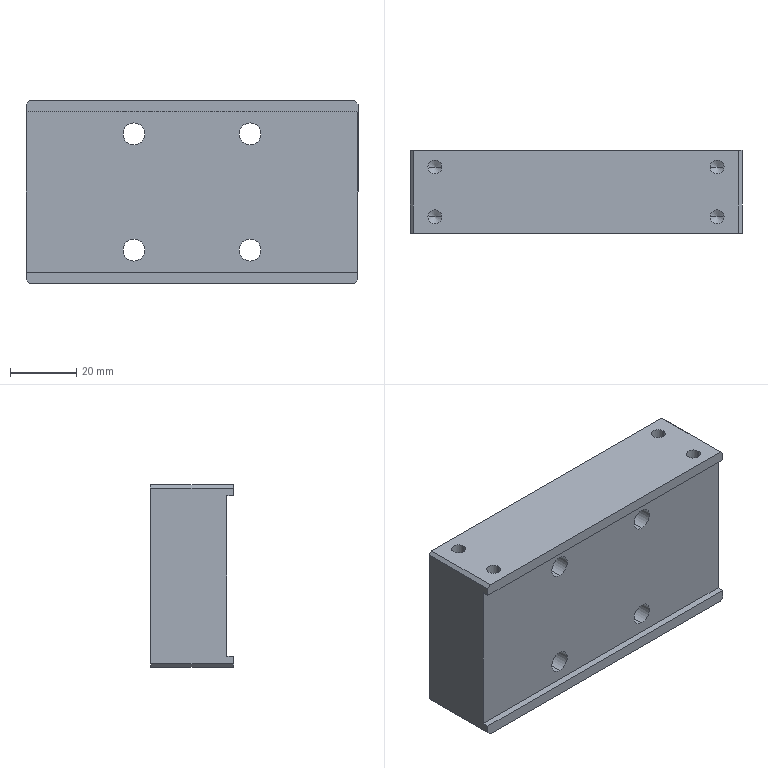Part | SolidWorks | features HoleWzd 4, Chamfer 1, Extrusion 1, ICE 1 | 1 solid | 82 faces | box 100 x 25 x 55 mm | volume 120725 mm3 | cylinder 40 | cone 24 | plane 18 | commonest cylinder face diameters 4.2 x20 6.6 x8 11 x8 5 x4